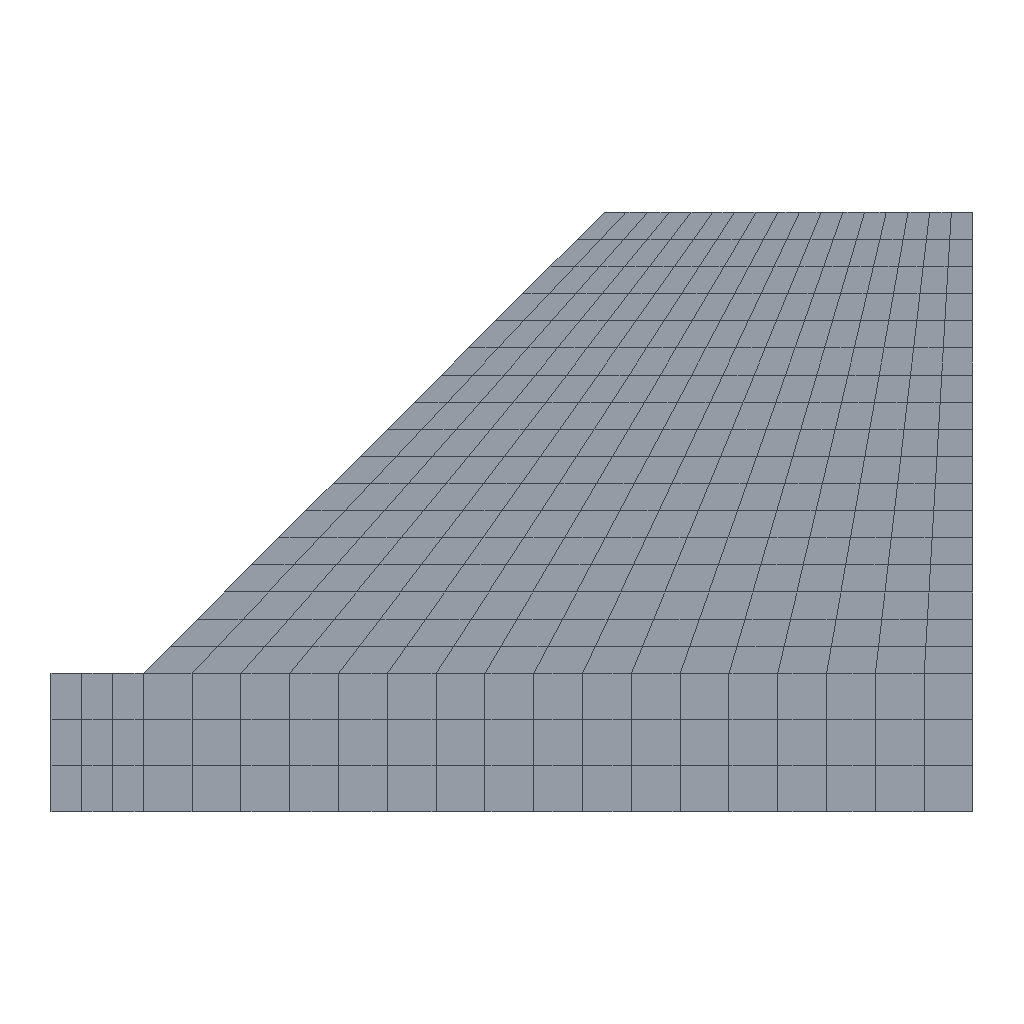Simulation study | abaqus
Set-up summary:
category,name,step,type,value,unit,region
solver,abaqus,,Abaqus/CAE 2024
units,mm-N-s-tonne (MPa),,inferred,E=100000 density=
analysis,Load,,static,time_period=1
analysis,Reduce,,static,time_period=1
mesh,nodes,,,390
mesh,elements,,,349
element_type,CPE4,,,349
material,soil,,E,100000
material,soil,,nu,0.35
material,soil,,behaviors,plastic; mohr coulomb; mohr coulomb hardening
section,soil,,solid section,,,_PickedSet3
load,,initial,initial condition field
load,Load-1,Load,by,-20,,_PickedSet6
bc,BC-1,initial,fixed,[dofs=x],,_PickedSet4
bc,BC-2,initial,fixed,"[dofs=x,y n=2]",,_PickedSet5
Abaqus input file, long lists of numbers shortened:
*Conflicts, Generated keywords
*Heading
** Job name: deck Model name: Model-1
** Generated by: Abaqus/CAE 2024
*Preprint, echo=NO, model=NO, history=NO, contact=NO
*Conflicts, User edited keywords
*Conflicts, End of conflict block
*Part, name=slope
*Node
      1,           2.,           0.
      2,           2.,           3.
** (388 more lines like these left out)
*Element, type=CPE4
 1,   1,   9,  99,  16
 2,   9,  10, 100,  99
** (347 more lines like these left out)
*Nset, nset=slope, generate
   1,  390,    1
*Elset, elset=slope, generate
   1,  349,    1
*Nset, nset=_PickedSet3, internal, generate
   1,  390,    1
*Elset, elset=_PickedSet3, internal, generate
   1,  349,    1
** Section: soil
*Solid Section, elset=_PickedSet3, material=soil
1.,
*End Part
**
**
** ASSEMBLY
**
*Assembly, name=Assembly
**
*Instance, name=slope-1, part=slope
*End Instance
**
*Nset, nset=_PickedSet4, internal, instance=slope-1
  3,  4,  5,  6,  7, 13, 14, 49, 50, 51, 52, 53, 54, 55, 56, 57
 58, 59, 60, 61, 62, 63, 64, 65, 66
*Elset, elset=_PickedSet4, internal, instance=slope-1
   7,   8,   9,  10,  27,  44,  77,  94, 111, 128, 145, 162, 179, 196, 213, 230
 247, 264, 281, 298, 315, 332, 349
*Nset, nset=_PickedSet5, internal, instance=slope-1
  1,  4,  6, 15, 16, 33, 34, 35, 36, 37, 38, 39, 40, 41, 42, 43
 44, 45, 46, 47, 48
*Elset, elset=_PickedSet5, internal, instance=slope-1
  1,  4,  7, 44, 45, 46, 47, 48, 49, 50, 51, 52, 53, 54, 55, 56
 57, 58, 59, 60
*Nset, nset=_PickedSet6, internal, instance=slope-1, generate
   1,  390,    1
*Elset, elset=_PickedSet6, internal, instance=slope-1, generate
   1,  349,    1
*End Assembly
**
** MATERIALS
**
*Material, name=soil
*Elastic
100000., 0.35
*Mohr Coulomb, dependencies=1
 36.052,   0., ,  0.5
  25.887,   0., , 0.75
     20.,   0., ,   1.
 16.234,   0., , 1.25
  13.639,   0., ,  1.5
  11.749,   0., , 1.75
 10.314,   0., ,   2.
*Mohr Coulomb Hardening, dependencies=1
   24.76,   0., ,  0.5
 16.507,   0., , 0.75
   12.38,   0., ,   1.
   9.904,   0., , 1.25
 8.253,   0., ,  1.5
 7.074,   0., , 1.75
    6.19,   0., ,   2.
**
** BOUNDARY CONDITIONS
**
** Name: BC-1 Type: Displacement/Rotation
*Boundary
_PickedSet4, 1, 1
** Name: BC-2 Type: Displacement/Rotation
*Boundary
_PickedSet5, 1, 1
_PickedSet5, 2, 2
** ----------------------------------------------------------------
*initial conditions,type=field,VARIABLE=1
slope-1.slope,0.5
**
** STEP: Load
**
*Step, name=Load, nlgeom=NO, unsymm=YES
*Static
0.1, 1., 1e-05, 1.
**
** LOADS
**
** Name: Load-1   Type: Body force
*Dload
_PickedSet6, BY, -20.
**
** OUTPUT REQUESTS
**
*Restart, write, frequency=0
*Print, solve=NO
**
** FIELD OUTPUT: F-Output-1
**
*Output, field
*Node Output
CF, RF, U
*Element Output, directions=YES
FV, LE, PE, PEEQ, PEMAG, S
*Contact Output
CDISP, CSTRESS
**
** HISTORY OUTPUT: H-Output-1
**
*Output, history, variable=PRESELECT
*End Step
** ----------------------------------------------------------------
**
** STEP: Reduce
**
*Step, name=Reduce, nlgeom=NO, unsymm=YES
*Static
0.1, 1., 1e-05, 1.
*field,VARIABLE=1
slope-1.slope,2
**
** OUTPUT REQUESTS
**
*Restart, write, frequency=0
**
** FIELD OUTPUT: F-Output-1
**
*Output, field
*Node Output
CF, RF, U
*Element Output, directions=YES
FV, LE, PE, PEEQ, PEMAG, S
*Contact Output
CDISP, CSTRESS
**
** HISTORY OUTPUT: H-Output-1
**
*Output, history, variable=PRESELECT
*End Step
Results summary:
result,odb.job_status,,,JOB_STATUS_EXITED_WITH_ERROR,"consistent, unstated (Abaqus has no unit system)"
result,steps[0].procedure,Load,,*STATIC,"consistent, unstated (Abaqus has no unit system)"
result,steps[0].time_period,Load,,1,"consistent, unstated (Abaqus has no unit system)"
result,steps[0].n_frames,Load,,7,"consistent, unstated (Abaqus has no unit system)"
result,steps[0].last_frame.id,Load,,6,"consistent, unstated (Abaqus has no unit system)"
result,steps[0].last_frame.value,Load,,1,"consistent, unstated (Abaqus has no unit system)"
result,steps[0].last_frame.description,Load,,Increment      6: Step Time =    1.000,"consistent, unstated (Abaqus has no unit system)"
result,steps[0].completed,Load,,True,"consistent, unstated (Abaqus has no unit system)"
result,steps[0].max_U_magnitude,Load,,0.01159,"consistent, unstated (Abaqus has no unit system)"
result,steps[0].max_S_mises,Load,,116.097,"consistent, unstated (Abaqus has no unit system)"
result,steps[0].RF_sum[1],Load,,3.52859e-05,"consistent, unstated (Abaqus has no unit system)"
result,steps[0].RF_sum[2],Load,,3800,"consistent, unstated (Abaqus has no unit system)"
result,steps[1].procedure,Reduce,,*STATIC,"consistent, unstated (Abaqus has no unit system)"
result,steps[1].time_period,Reduce,,0.3718,"consistent, unstated (Abaqus has no unit system)"
result,steps[1].n_frames,Reduce,,57,"consistent, unstated (Abaqus has no unit system)"
result,steps[1].last_frame.id,Reduce,,56,"consistent, unstated (Abaqus has no unit system)"
result,steps[1].last_frame.value,Reduce,,0.3718,"consistent, unstated (Abaqus has no unit system)"
result,steps[1].last_frame.description,Reduce,,Increment     56: Step Time =   0.3718,"consistent, unstated (Abaqus has no unit system)"
result,steps[1].completed,Reduce,,True,"consistent, unstated (Abaqus has no unit system)"
result,steps[1].max_U_magnitude,Reduce,,5.268,"consistent, unstated (Abaqus has no unit system)"
result,steps[1].max_S_mises,Reduce,,126.379,"consistent, unstated (Abaqus has no unit system)"
result,steps[1].RF_sum[1],Reduce,,-0.0001655,"consistent, unstated (Abaqus has no unit system)"
result,steps[1].RF_sum[2],Reduce,,3800,"consistent, unstated (Abaqus has no unit system)"